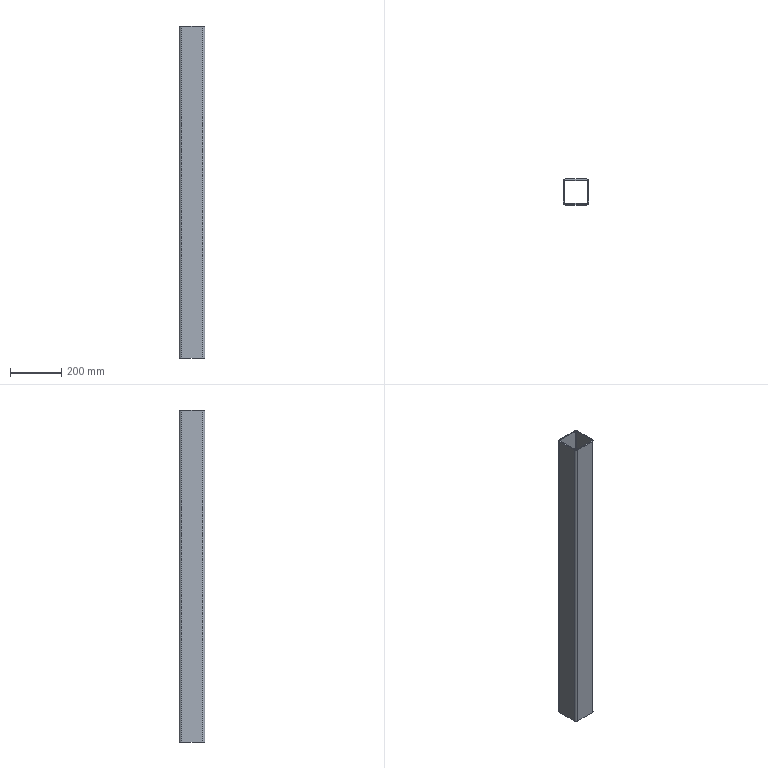Part | SolidWorks | features Extrusion 1 | 1 solid | 18 faces | box 100 x 100 x 1290 mm | volume 2367949 mm3 | plane 10 | cylinder 8 | commonest cylinder face diameters 10 x4 20 x4
STEP:
#1=CARTESIAN_POINT('',(-40.,50.,645.));
#2=VERTEX_POINT('',#1);
#3=CARTESIAN_POINT('',(-50.,40.,645.));
#4=VERTEX_POINT('',#3);
#5=CARTESIAN_POINT('',(-40.,40.,645.));
#6=DIRECTION('',(0.,0.,1.));
#7=DIRECTION('',(1.,0.,0.));
#8=AXIS2_PLACEMENT_3D('',#5,#6,#7);
#9=CIRCLE('',#8,10.);
#10=EDGE_CURVE('',#2,#4,#9,.T.);
#11=ORIENTED_EDGE('',*,*,#10,.T.);
#12=CARTESIAN_POINT('',(-50.,-40.,645.));
#13=VERTEX_POINT('',#12);
#14=CARTESIAN_POINT('',(-50.,40.,645.));
#15=DIRECTION('',(0.,-1.,0.));
#16=VECTOR('',#15,1000.);
#17=LINE('',#14,#16);
#18=EDGE_CURVE('',#4,#13,#17,.T.);
#19=ORIENTED_EDGE('',*,*,#18,.T.);
#20=CARTESIAN_POINT('',(-40.,-50.,645.));
#21=VERTEX_POINT('',#20);
#22=CARTESIAN_POINT('',(-40.,-40.,645.));
#23=DIRECTION('',(0.,0.,1.));
#24=DIRECTION('',(-1.,0.,0.));
#25=AXIS2_PLACEMENT_3D('',#22,#23,#24);
#26=CIRCLE('',#25,10.);
#27=EDGE_CURVE('',#13,#21,#26,.T.);
#28=ORIENTED_EDGE('',*,*,#27,.T.);
#29=CARTESIAN_POINT('',(40.,-50.,645.));
#30=VERTEX_POINT('',#29);
#31=CARTESIAN_POINT('',(40.,-50.,645.));
#32=DIRECTION('',(1.,0.,0.));
#33=VECTOR('',#32,1000.);
#34=LINE('',#31,#33);
#35=EDGE_CURVE('',#21,#30,#34,.T.);
#36=ORIENTED_EDGE('',*,*,#35,.T.);
#37=CARTESIAN_POINT('',(50.,-40.,645.));
#38=VERTEX_POINT('',#37);
#39=CARTESIAN_POINT('',(40.,-40.,645.));
#40=DIRECTION('',(0.,0.,1.));
#41=DIRECTION('',(1.,0.,0.));
#42=AXIS2_PLACEMENT_3D('',#39,#40,#41);
#43=CIRCLE('',#42,10.);
#44=EDGE_CURVE('',#30,#38,#43,.T.);
#45=ORIENTED_EDGE('',*,*,#44,.T.);
#46=CARTESIAN_POINT('',(50.,40.,645.));
#47=VERTEX_POINT('',#46);
#48=CARTESIAN_POINT('',(50.,-40.,645.));
#49=DIRECTION('',(0.,1.,0.));
#50=VECTOR('',#49,1000.);
#51=LINE('',#48,#50);
#52=EDGE_CURVE('',#38,#47,#51,.T.);
#53=ORIENTED_EDGE('',*,*,#52,.T.);
#54=CARTESIAN_POINT('',(40.,50.,645.));
#55=VERTEX_POINT('',#54);
#56=CARTESIAN_POINT('',(40.,40.,645.));
#57=DIRECTION('',(0.,0.,1.));
#58=DIRECTION('',(-1.,0.,0.));
#59=AXIS2_PLACEMENT_3D('',#56,#57,#58);
#60=CIRCLE('',#59,10.);
#61=EDGE_CURVE('',#47,#55,#60,.T.);
#62=ORIENTED_EDGE('',*,*,#61,.T.);
#63=CARTESIAN_POINT('',(0.,50.,645.));
#64=DIRECTION('',(-1.,0.,0.));
#65=VECTOR('',#64,1000.);
#66=LINE('',#63,#65);
#67=EDGE_CURVE('',#55,#2,#66,.T.);
#68=ORIENTED_EDGE('',*,*,#67,.T.);
#69=EDGE_LOOP('',(#11,#19,#28,#36,#45,#53,#62,#68));
#70=FACE_OUTER_BOUND('',#69,.T.);
#71=CARTESIAN_POINT('',(-45.,40.,645.));
#72=VERTEX_POINT('',#71);
#73=CARTESIAN_POINT('',(-45.,-40.,645.));
#74=VERTEX_POINT('',#73);
#75=CARTESIAN_POINT('',(-45.,40.,645.));
#76=DIRECTION('',(0.,-1.,0.));
#77=VECTOR('',#76,1000.);
#78=LINE('',#75,#77);
#79=EDGE_CURVE('',#72,#74,#78,.T.);
#80=ORIENTED_EDGE('',*,*,#79,.F.);
#81=CARTESIAN_POINT('',(-40.,45.,645.));
#82=VERTEX_POINT('',#81);
#83=CARTESIAN_POINT('',(-40.,40.,645.));
#84=DIRECTION('',(0.,0.,1.));
#85=DIRECTION('',(1.,0.,0.));
#86=AXIS2_PLACEMENT_3D('',#83,#84,#85);
#87=CIRCLE('',#86,5.);
#88=EDGE_CURVE('',#82,#72,#87,.T.);
#89=ORIENTED_EDGE('',*,*,#88,.F.);
#90=CARTESIAN_POINT('',(40.,45.,645.));
#91=VERTEX_POINT('',#90);
#92=CARTESIAN_POINT('',(0.,45.,645.));
#93=DIRECTION('',(-1.,0.,0.));
#94=VECTOR('',#93,1000.);
#95=LINE('',#92,#94);
#96=EDGE_CURVE('',#91,#82,#95,.T.);
#97=ORIENTED_EDGE('',*,*,#96,.F.);
#98=CARTESIAN_POINT('',(45.,40.,645.));
#99=VERTEX_POINT('',#98);
#100=CARTESIAN_POINT('',(40.,40.,645.));
#101=DIRECTION('',(0.,0.,1.));
#102=DIRECTION('',(-1.,0.,0.));
#103=AXIS2_PLACEMENT_3D('',#100,#101,#102);
#104=CIRCLE('',#103,5.);
#105=EDGE_CURVE('',#99,#91,#104,.T.);
#106=ORIENTED_EDGE('',*,*,#105,.F.);
#107=CARTESIAN_POINT('',(45.,-40.,645.));
#108=VERTEX_POINT('',#107);
#109=CARTESIAN_POINT('',(45.,-40.,645.));
#110=DIRECTION('',(0.,1.,0.));
#111=VECTOR('',#110,1000.);
#112=LINE('',#109,#111);
#113=EDGE_CURVE('',#108,#99,#112,.T.);
#114=ORIENTED_EDGE('',*,*,#113,.F.);
#115=CARTESIAN_POINT('',(40.,-45.,645.));
#116=VERTEX_POINT('',#115);
#117=CARTESIAN_POINT('',(40.,-40.,645.));
#118=DIRECTION('',(0.,0.,1.));
#119=DIRECTION('',(1.,0.,0.));
#120=AXIS2_PLACEMENT_3D('',#117,#118,#119);
#121=CIRCLE('',#120,5.);
#122=EDGE_CURVE('',#116,#108,#121,.T.);
#123=ORIENTED_EDGE('',*,*,#122,.F.);
#124=CARTESIAN_POINT('',(-40.,-45.,645.));
#125=VERTEX_POINT('',#124);
#126=CARTESIAN_POINT('',(40.,-45.,645.));
#127=DIRECTION('',(1.,0.,0.));
#128=VECTOR('',#127,1000.);
#129=LINE('',#126,#128);
#130=EDGE_CURVE('',#125,#116,#129,.T.);
#131=ORIENTED_EDGE('',*,*,#130,.F.);
#132=CARTESIAN_POINT('',(-40.,-40.,645.));
#133=DIRECTION('',(0.,0.,1.));
#134=DIRECTION('',(-1.,0.,0.));
#135=AXIS2_PLACEMENT_3D('',#132,#133,#134);
#136=CIRCLE('',#135,5.);
#137=EDGE_CURVE('',#74,#125,#136,.T.);
#138=ORIENTED_EDGE('',*,*,#137,.F.);
#139=EDGE_LOOP('',(#80,#89,#97,#106,#114,#123,#131,#138));
#140=FACE_BOUND('',#139,.T.);
#141=CARTESIAN_POINT('',(-40.,40.,645.));
#142=DIRECTION('',(0.,0.,1.));
#143=DIRECTION('',(1.,0.,0.));
#144=AXIS2_PLACEMENT_3D('',#141,#142,#143);
#145=PLANE('',#144);
#146=ADVANCED_FACE('',(#70,#140),#145,.T.);
#147=CARTESIAN_POINT('',(-40.,50.,-645.));
#148=VERTEX_POINT('',#147);
#149=CARTESIAN_POINT('',(-50.,40.,-645.));
#150=VERTEX_POINT('',#149);
#151=CARTESIAN_POINT('',(-40.,40.,-645.));
#152=DIRECTION('',(0.,0.,1.));
#153=DIRECTION('',(1.,0.,0.));
#154=AXIS2_PLACEMENT_3D('',#151,#152,#153);
#155=CIRCLE('',#154,10.);
#156=EDGE_CURVE('',#148,#150,#155,.T.);
#157=ORIENTED_EDGE('',*,*,#156,.F.);
#158=CARTESIAN_POINT('',(40.,50.,-645.));
#159=VERTEX_POINT('',#158);
#160=CARTESIAN_POINT('',(0.,50.,-645.));
#161=DIRECTION('',(-1.,0.,0.));
#162=VECTOR('',#161,1000.);
#163=LINE('',#160,#162);
#164=EDGE_CURVE('',#159,#148,#163,.T.);
#165=ORIENTED_EDGE('',*,*,#164,.F.);
#166=CARTESIAN_POINT('',(50.,40.,-645.));
#167=VERTEX_POINT('',#166);
#168=CARTESIAN_POINT('',(40.,40.,-645.));
#169=DIRECTION('',(0.,0.,1.));
#170=DIRECTION('',(-1.,0.,0.));
#171=AXIS2_PLACEMENT_3D('',#168,#169,#170);
#172=CIRCLE('',#171,10.);
#173=EDGE_CURVE('',#167,#159,#172,.T.);
#174=ORIENTED_EDGE('',*,*,#173,.F.);
#175=CARTESIAN_POINT('',(50.,-40.,-645.));
#176=VERTEX_POINT('',#175);
#177=CARTESIAN_POINT('',(50.,40.,-645.));
#178=DIRECTION('',(0.,1.,0.));
#179=VECTOR('',#178,1000.);
#180=LINE('',#177,#179);
#181=EDGE_CURVE('',#176,#167,#180,.T.);
#182=ORIENTED_EDGE('',*,*,#181,.F.);
#183=CARTESIAN_POINT('',(40.,-50.,-645.));
#184=VERTEX_POINT('',#183);
#185=CARTESIAN_POINT('',(40.,-40.,-645.));
#186=DIRECTION('',(0.,0.,1.));
#187=DIRECTION('',(1.,0.,0.));
#188=AXIS2_PLACEMENT_3D('',#185,#186,#187);
#189=CIRCLE('',#188,10.);
#190=EDGE_CURVE('',#184,#176,#189,.T.);
#191=ORIENTED_EDGE('',*,*,#190,.F.);
#192=CARTESIAN_POINT('',(-40.,-50.,-645.));
#193=VERTEX_POINT('',#192);
#194=CARTESIAN_POINT('',(40.,-50.,-645.));
#195=DIRECTION('',(1.,0.,0.));
#196=VECTOR('',#195,1000.);
#197=LINE('',#194,#196);
#198=EDGE_CURVE('',#193,#184,#197,.T.);
#199=ORIENTED_EDGE('',*,*,#198,.F.);
#200=CARTESIAN_POINT('',(-50.,-40.,-645.));
#201=VERTEX_POINT('',#200);
#202=CARTESIAN_POINT('',(-40.,-40.,-645.));
#203=DIRECTION('',(0.,0.,1.));
#204=DIRECTION('',(-1.,0.,0.));
#205=AXIS2_PLACEMENT_3D('',#202,#203,#204);
#206=CIRCLE('',#205,10.);
#207=EDGE_CURVE('',#201,#193,#206,.T.);
#208=ORIENTED_EDGE('',*,*,#207,.F.);
#209=CARTESIAN_POINT('',(-50.,-40.,-645.));
#210=DIRECTION('',(0.,-1.,0.));
#211=VECTOR('',#210,1000.);
#212=LINE('',#209,#211);
#213=EDGE_CURVE('',#150,#201,#212,.T.);
#214=ORIENTED_EDGE('',*,*,#213,.F.);
#215=EDGE_LOOP('',(#157,#165,#174,#182,#191,#199,#208,#214));
#216=FACE_OUTER_BOUND('',#215,.T.);
#217=CARTESIAN_POINT('',(-40.,45.,-645.));
#218=VERTEX_POINT('',#217);
#219=CARTESIAN_POINT('',(-45.,40.,-645.));
#220=VERTEX_POINT('',#219);
#221=CARTESIAN_POINT('',(-40.,40.,-645.));
#222=DIRECTION('',(0.,0.,1.));
#223=DIRECTION('',(1.,0.,0.));
#224=AXIS2_PLACEMENT_3D('',#221,#222,#223);
#225=CIRCLE('',#224,5.);
#226=EDGE_CURVE('',#218,#220,#225,.T.);
#227=ORIENTED_EDGE('',*,*,#226,.T.);
#228=CARTESIAN_POINT('',(-45.,-40.,-645.));
#229=VERTEX_POINT('',#228);
#230=CARTESIAN_POINT('',(-45.,-40.,-645.));
#231=DIRECTION('',(0.,-1.,0.));
#232=VECTOR('',#231,1000.);
#233=LINE('',#230,#232);
#234=EDGE_CURVE('',#220,#229,#233,.T.);
#235=ORIENTED_EDGE('',*,*,#234,.T.);
#236=CARTESIAN_POINT('',(-40.,-45.,-645.));
#237=VERTEX_POINT('',#236);
#238=CARTESIAN_POINT('',(-40.,-40.,-645.));
#239=DIRECTION('',(0.,0.,1.));
#240=DIRECTION('',(-1.,0.,0.));
#241=AXIS2_PLACEMENT_3D('',#238,#239,#240);
#242=CIRCLE('',#241,5.);
#243=EDGE_CURVE('',#229,#237,#242,.T.);
#244=ORIENTED_EDGE('',*,*,#243,.T.);
#245=CARTESIAN_POINT('',(40.,-45.,-645.));
#246=VERTEX_POINT('',#245);
#247=CARTESIAN_POINT('',(40.,-45.,-645.));
#248=DIRECTION('',(1.,0.,0.));
#249=VECTOR('',#248,1000.);
#250=LINE('',#247,#249);
#251=EDGE_CURVE('',#237,#246,#250,.T.);
#252=ORIENTED_EDGE('',*,*,#251,.T.);
#253=CARTESIAN_POINT('',(45.,-40.,-645.));
#254=VERTEX_POINT('',#253);
#255=CARTESIAN_POINT('',(40.,-40.,-645.));
#256=DIRECTION('',(0.,0.,1.));
#257=DIRECTION('',(1.,0.,0.));
#258=AXIS2_PLACEMENT_3D('',#255,#256,#257);
#259=CIRCLE('',#258,5.);
#260=EDGE_CURVE('',#246,#254,#259,.T.);
#261=ORIENTED_EDGE('',*,*,#260,.T.);
#262=CARTESIAN_POINT('',(45.,40.,-645.));
#263=VERTEX_POINT('',#262);
#264=CARTESIAN_POINT('',(45.,40.,-645.));
#265=DIRECTION('',(0.,1.,0.));
#266=VECTOR('',#265,1000.);
#267=LINE('',#264,#266);
#268=EDGE_CURVE('',#254,#263,#267,.T.);
#269=ORIENTED_EDGE('',*,*,#268,.T.);
#270=CARTESIAN_POINT('',(40.,45.,-645.));
#271=VERTEX_POINT('',#270);
#272=CARTESIAN_POINT('',(40.,40.,-645.));
#273=DIRECTION('',(0.,0.,1.));
#274=DIRECTION('',(-1.,0.,0.));
#275=AXIS2_PLACEMENT_3D('',#272,#273,#274);
#276=CIRCLE('',#275,5.);
#277=EDGE_CURVE('',#263,#271,#276,.T.);
#278=ORIENTED_EDGE('',*,*,#277,.T.);
#279=CARTESIAN_POINT('',(0.,45.,-645.));
#280=DIRECTION('',(-1.,0.,0.));
#281=VECTOR('',#280,1000.);
#282=LINE('',#279,#281);
#283=EDGE_CURVE('',#271,#218,#282,.T.);
#284=ORIENTED_EDGE('',*,*,#283,.T.);
#285=EDGE_LOOP('',(#227,#235,#244,#252,#261,#269,#278,#284));
#286=FACE_BOUND('',#285,.T.);
#287=CARTESIAN_POINT('',(-40.,40.,-645.));
#288=DIRECTION('',(0.,0.,1.));
#289=DIRECTION('',(1.,0.,0.));
#290=AXIS2_PLACEMENT_3D('',#287,#288,#289);
#291=PLANE('',#290);
#292=ADVANCED_FACE('',(#216,#286),#291,.F.);
#293=ORIENTED_EDGE('',*,*,#156,.T.);
#294=CARTESIAN_POINT('',(-50.,40.,645.));
#295=DIRECTION('',(0.,0.,-1.));
#296=VECTOR('',#295,1000.);
#297=LINE('',#294,#296);
#298=EDGE_CURVE('',#4,#150,#297,.T.);
#299=ORIENTED_EDGE('',*,*,#298,.F.);
#300=ORIENTED_EDGE('',*,*,#10,.F.);
#301=CARTESIAN_POINT('',(-40.,50.,645.));
#302=DIRECTION('',(0.,0.,-1.));
#303=VECTOR('',#302,1000.);
#304=LINE('',#301,#303);
#305=EDGE_CURVE('',#2,#148,#304,.T.);
#306=ORIENTED_EDGE('',*,*,#305,.T.);
#307=EDGE_LOOP('',(#293,#299,#300,#306));
#308=FACE_OUTER_BOUND('',#307,.T.);
#309=CARTESIAN_POINT('',(-40.,40.,645.));
#310=DIRECTION('',(0.,0.,-1.));
#311=DIRECTION('',(-1.,0.,0.));
#312=AXIS2_PLACEMENT_3D('',#309,#310,#311);
#313=CYLINDRICAL_SURFACE('',#312,10.);
#314=ADVANCED_FACE('',(#308),#313,.T.);
#315=ORIENTED_EDGE('',*,*,#213,.T.);
#316=CARTESIAN_POINT('',(-50.,-40.,645.));
#317=DIRECTION('',(0.,0.,-1.));
#318=VECTOR('',#317,1000.);
#319=LINE('',#316,#318);
#320=EDGE_CURVE('',#13,#201,#319,.T.);
#321=ORIENTED_EDGE('',*,*,#320,.F.);
#322=ORIENTED_EDGE('',*,*,#18,.F.);
#323=ORIENTED_EDGE('',*,*,#298,.T.);
#324=EDGE_LOOP('',(#315,#321,#322,#323));
#325=FACE_OUTER_BOUND('',#324,.T.);
#326=CARTESIAN_POINT('',(-50.,-40.,645.));
#327=DIRECTION('',(1.,0.,0.));
#328=DIRECTION('',(0.,0.,-1.));
#329=AXIS2_PLACEMENT_3D('',#326,#327,#328);
#330=PLANE('',#329);
#331=ADVANCED_FACE('',(#325),#330,.F.);
#332=ORIENTED_EDGE('',*,*,#207,.T.);
#333=CARTESIAN_POINT('',(-40.,-50.,645.));
#334=DIRECTION('',(0.,0.,-1.));
#335=VECTOR('',#334,1000.);
#336=LINE('',#333,#335);
#337=EDGE_CURVE('',#21,#193,#336,.T.);
#338=ORIENTED_EDGE('',*,*,#337,.F.);
#339=ORIENTED_EDGE('',*,*,#27,.F.);
#340=ORIENTED_EDGE('',*,*,#320,.T.);
#341=EDGE_LOOP('',(#332,#338,#339,#340));
#342=FACE_OUTER_BOUND('',#341,.T.);
#343=CARTESIAN_POINT('',(-40.,-40.,645.));
#344=DIRECTION('',(0.,0.,-1.));
#345=DIRECTION('',(-1.,0.,0.));
#346=AXIS2_PLACEMENT_3D('',#343,#344,#345);
#347=CYLINDRICAL_SURFACE('',#346,10.);
#348=ADVANCED_FACE('',(#342),#347,.T.);
#349=ORIENTED_EDGE('',*,*,#198,.T.);
#350=CARTESIAN_POINT('',(40.,-50.,645.));
#351=DIRECTION('',(0.,0.,-1.));
#352=VECTOR('',#351,1000.);
#353=LINE('',#350,#352);
#354=EDGE_CURVE('',#30,#184,#353,.T.);
#355=ORIENTED_EDGE('',*,*,#354,.F.);
#356=ORIENTED_EDGE('',*,*,#35,.F.);
#357=ORIENTED_EDGE('',*,*,#337,.T.);
#358=EDGE_LOOP('',(#349,#355,#356,#357));
#359=FACE_OUTER_BOUND('',#358,.T.);
#360=CARTESIAN_POINT('',(40.,-50.,645.));
#361=DIRECTION('',(0.,1.,0.));
#362=DIRECTION('',(-1.,0.,0.));
#363=AXIS2_PLACEMENT_3D('',#360,#361,#362);
#364=PLANE('',#363);
#365=ADVANCED_FACE('',(#359),#364,.F.);
#366=ORIENTED_EDGE('',*,*,#190,.T.);
#367=CARTESIAN_POINT('',(50.,-40.,645.));
#368=DIRECTION('',(0.,0.,-1.));
#369=VECTOR('',#368,1000.);
#370=LINE('',#367,#369);
#371=EDGE_CURVE('',#38,#176,#370,.T.);
#372=ORIENTED_EDGE('',*,*,#371,.F.);
#373=ORIENTED_EDGE('',*,*,#44,.F.);
#374=ORIENTED_EDGE('',*,*,#354,.T.);
#375=EDGE_LOOP('',(#366,#372,#373,#374));
#376=FACE_OUTER_BOUND('',#375,.T.);
#377=CARTESIAN_POINT('',(40.,-40.,645.));
#378=DIRECTION('',(0.,0.,-1.));
#379=DIRECTION('',(-1.,0.,0.));
#380=AXIS2_PLACEMENT_3D('',#377,#378,#379);
#381=CYLINDRICAL_SURFACE('',#380,10.);
#382=ADVANCED_FACE('',(#376),#381,.T.);
#383=ORIENTED_EDGE('',*,*,#181,.T.);
#384=CARTESIAN_POINT('',(50.,40.,645.));
#385=DIRECTION('',(0.,0.,-1.));
#386=VECTOR('',#385,1000.);
#387=LINE('',#384,#386);
#388=EDGE_CURVE('',#47,#167,#387,.T.);
#389=ORIENTED_EDGE('',*,*,#388,.F.);
#390=ORIENTED_EDGE('',*,*,#52,.F.);
#391=ORIENTED_EDGE('',*,*,#371,.T.);
#392=EDGE_LOOP('',(#383,#389,#390,#391));
#393=FACE_OUTER_BOUND('',#392,.T.);
#394=CARTESIAN_POINT('',(50.,40.,645.));
#395=DIRECTION('',(-1.,0.,0.));
#396=DIRECTION('',(0.,0.,1.));
#397=AXIS2_PLACEMENT_3D('',#394,#395,#396);
#398=PLANE('',#397);
#399=ADVANCED_FACE('',(#393),#398,.F.);
#400=ORIENTED_EDGE('',*,*,#173,.T.);
#401=CARTESIAN_POINT('',(40.,50.,645.));
#402=DIRECTION('',(0.,0.,-1.));
#403=VECTOR('',#402,1000.);
#404=LINE('',#401,#403);
#405=EDGE_CURVE('',#55,#159,#404,.T.);
#406=ORIENTED_EDGE('',*,*,#405,.F.);
#407=ORIENTED_EDGE('',*,*,#61,.F.);
#408=ORIENTED_EDGE('',*,*,#388,.T.);
#409=EDGE_LOOP('',(#400,#406,#407,#408));
#410=FACE_OUTER_BOUND('',#409,.T.);
#411=CARTESIAN_POINT('',(40.,40.,645.));
#412=DIRECTION('',(0.,0.,-1.));
#413=DIRECTION('',(-1.,0.,0.));
#414=AXIS2_PLACEMENT_3D('',#411,#412,#413);
#415=CYLINDRICAL_SURFACE('',#414,10.);
#416=ADVANCED_FACE('',(#410),#415,.T.);
#417=ORIENTED_EDGE('',*,*,#164,.T.);
#418=ORIENTED_EDGE('',*,*,#305,.F.);
#419=ORIENTED_EDGE('',*,*,#67,.F.);
#420=ORIENTED_EDGE('',*,*,#405,.T.);
#421=EDGE_LOOP('',(#417,#418,#419,#420));
#422=FACE_OUTER_BOUND('',#421,.T.);
#423=CARTESIAN_POINT('',(0.,50.,645.));
#424=DIRECTION('',(0.,-1.,0.));
#425=DIRECTION('',(0.,0.,-1.));
#426=AXIS2_PLACEMENT_3D('',#423,#424,#425);
#427=PLANE('',#426);
#428=ADVANCED_FACE('',(#422),#427,.F.);
#429=ORIENTED_EDGE('',*,*,#226,.F.);
#430=CARTESIAN_POINT('',(-40.,45.,645.));
#431=DIRECTION('',(0.,0.,-1.));
#432=VECTOR('',#431,1000.);
#433=LINE('',#430,#432);
#434=EDGE_CURVE('',#82,#218,#433,.T.);
#435=ORIENTED_EDGE('',*,*,#434,.F.);
#436=ORIENTED_EDGE('',*,*,#88,.T.);
#437=CARTESIAN_POINT('',(-45.,40.,645.));
#438=DIRECTION('',(0.,0.,-1.));
#439=VECTOR('',#438,1000.);
#440=LINE('',#437,#439);
#441=EDGE_CURVE('',#72,#220,#440,.T.);
#442=ORIENTED_EDGE('',*,*,#441,.T.);
#443=EDGE_LOOP('',(#429,#435,#436,#442));
#444=FACE_OUTER_BOUND('',#443,.T.);
#445=CARTESIAN_POINT('',(-40.,40.,645.));
#446=DIRECTION('',(0.,0.,-1.));
#447=DIRECTION('',(-1.,0.,0.));
#448=AXIS2_PLACEMENT_3D('',#445,#446,#447);
#449=CYLINDRICAL_SURFACE('',#448,5.);
#450=ADVANCED_FACE('',(#444),#449,.F.);
#451=ORIENTED_EDGE('',*,*,#234,.F.);
#452=ORIENTED_EDGE('',*,*,#441,.F.);
#453=ORIENTED_EDGE('',*,*,#79,.T.);
#454=CARTESIAN_POINT('',(-45.,-40.,645.));
#455=DIRECTION('',(0.,0.,-1.));
#456=VECTOR('',#455,1000.);
#457=LINE('',#454,#456);
#458=EDGE_CURVE('',#74,#229,#457,.T.);
#459=ORIENTED_EDGE('',*,*,#458,.T.);
#460=EDGE_LOOP('',(#451,#452,#453,#459));
#461=FACE_OUTER_BOUND('',#460,.T.);
#462=CARTESIAN_POINT('',(-45.,-40.,645.));
#463=DIRECTION('',(1.,0.,0.));
#464=DIRECTION('',(0.,1.,0.));
#465=AXIS2_PLACEMENT_3D('',#462,#463,#464);
#466=PLANE('',#465);
#467=ADVANCED_FACE('',(#461),#466,.T.);
#468=ORIENTED_EDGE('',*,*,#243,.F.);
#469=ORIENTED_EDGE('',*,*,#458,.F.);
#470=ORIENTED_EDGE('',*,*,#137,.T.);
#471=CARTESIAN_POINT('',(-40.,-45.,645.));
#472=DIRECTION('',(0.,0.,-1.));
#473=VECTOR('',#472,1000.);
#474=LINE('',#471,#473);
#475=EDGE_CURVE('',#125,#237,#474,.T.);
#476=ORIENTED_EDGE('',*,*,#475,.T.);
#477=EDGE_LOOP('',(#468,#469,#470,#476));
#478=FACE_OUTER_BOUND('',#477,.T.);
#479=CARTESIAN_POINT('',(-40.,-40.,645.));
#480=DIRECTION('',(0.,0.,-1.));
#481=DIRECTION('',(-1.,0.,0.));
#482=AXIS2_PLACEMENT_3D('',#479,#480,#481);
#483=CYLINDRICAL_SURFACE('',#482,5.);
#484=ADVANCED_FACE('',(#478),#483,.F.);
#485=ORIENTED_EDGE('',*,*,#251,.F.);
#486=ORIENTED_EDGE('',*,*,#475,.F.);
#487=ORIENTED_EDGE('',*,*,#130,.T.);
#488=CARTESIAN_POINT('',(40.,-45.,645.));
#489=DIRECTION('',(0.,0.,-1.));
#490=VECTOR('',#489,1000.);
#491=LINE('',#488,#490);
#492=EDGE_CURVE('',#116,#246,#491,.T.);
#493=ORIENTED_EDGE('',*,*,#492,.T.);
#494=EDGE_LOOP('',(#485,#486,#487,#493));
#495=FACE_OUTER_BOUND('',#494,.T.);
#496=CARTESIAN_POINT('',(40.,-45.,645.));
#497=DIRECTION('',(0.,1.,0.));
#498=DIRECTION('',(-1.,0.,0.));
#499=AXIS2_PLACEMENT_3D('',#496,#497,#498);
#500=PLANE('',#499);
#501=ADVANCED_FACE('',(#495),#500,.T.);
#502=ORIENTED_EDGE('',*,*,#260,.F.);
#503=ORIENTED_EDGE('',*,*,#492,.F.);
#504=ORIENTED_EDGE('',*,*,#122,.T.);
#505=CARTESIAN_POINT('',(45.,-40.,645.));
#506=DIRECTION('',(0.,0.,-1.));
#507=VECTOR('',#506,1000.);
#508=LINE('',#505,#507);
#509=EDGE_CURVE('',#108,#254,#508,.T.);
#510=ORIENTED_EDGE('',*,*,#509,.T.);
#511=EDGE_LOOP('',(#502,#503,#504,#510));
#512=FACE_OUTER_BOUND('',#511,.T.);
#513=CARTESIAN_POINT('',(40.,-40.,645.));
#514=DIRECTION('',(0.,0.,-1.));
#515=DIRECTION('',(-1.,0.,0.));
#516=AXIS2_PLACEMENT_3D('',#513,#514,#515);
#517=CYLINDRICAL_SURFACE('',#516,5.);
#518=ADVANCED_FACE('',(#512),#517,.F.);
#519=ORIENTED_EDGE('',*,*,#268,.F.);
#520=ORIENTED_EDGE('',*,*,#509,.F.);
#521=ORIENTED_EDGE('',*,*,#113,.T.);
#522=CARTESIAN_POINT('',(45.,40.,645.));
#523=DIRECTION('',(0.,0.,-1.));
#524=VECTOR('',#523,1000.);
#525=LINE('',#522,#524);
#526=EDGE_CURVE('',#99,#263,#525,.T.);
#527=ORIENTED_EDGE('',*,*,#526,.T.);
#528=EDGE_LOOP('',(#519,#520,#521,#527));
#529=FACE_OUTER_BOUND('',#528,.T.);
#530=CARTESIAN_POINT('',(45.,40.,645.));
#531=DIRECTION('',(-1.,0.,0.));
#532=DIRECTION('',(0.,0.,1.));
#533=AXIS2_PLACEMENT_3D('',#530,#531,#532);
#534=PLANE('',#533);
#535=ADVANCED_FACE('',(#529),#534,.T.);
#536=ORIENTED_EDGE('',*,*,#277,.F.);
#537=ORIENTED_EDGE('',*,*,#526,.F.);
#538=ORIENTED_EDGE('',*,*,#105,.T.);
#539=CARTESIAN_POINT('',(40.,45.,645.));
#540=DIRECTION('',(0.,0.,-1.));
#541=VECTOR('',#540,1000.);
#542=LINE('',#539,#541);
#543=EDGE_CURVE('',#91,#271,#542,.T.);
#544=ORIENTED_EDGE('',*,*,#543,.T.);
#545=EDGE_LOOP('',(#536,#537,#538,#544));
#546=FACE_OUTER_BOUND('',#545,.T.);
#547=CARTESIAN_POINT('',(40.,40.,645.));
#548=DIRECTION('',(0.,0.,-1.));
#549=DIRECTION('',(-1.,0.,0.));
#550=AXIS2_PLACEMENT_3D('',#547,#548,#549);
#551=CYLINDRICAL_SURFACE('',#550,5.);
#552=ADVANCED_FACE('',(#546),#551,.F.);
#553=ORIENTED_EDGE('',*,*,#283,.F.);
#554=ORIENTED_EDGE('',*,*,#543,.F.);
#555=ORIENTED_EDGE('',*,*,#96,.T.);
#556=ORIENTED_EDGE('',*,*,#434,.T.);
#557=EDGE_LOOP('',(#553,#554,#555,#556));
#558=FACE_OUTER_BOUND('',#557,.T.);
#559=CARTESIAN_POINT('',(0.,45.,645.));
#560=DIRECTION('',(0.,-1.,0.));
#561=DIRECTION('',(1.,0.,0.));
#562=AXIS2_PLACEMENT_3D('',#559,#560,#561);
#563=PLANE('',#562);
#564=ADVANCED_FACE('',(#558),#563,.T.);
#565=CLOSED_SHELL('',(#146,#292,#314,#331,#348,#365,#382,#399,#416,#428,#450,#467,#484,#501,#518,#535,#552,#564));
#566=MANIFOLD_SOLID_BREP('',#565);
#567=CARTESIAN_POINT('',(0.,0.,0.));
#568=DIRECTION('',(0.,0.,1.));
#569=DIRECTION('',(1.,0.,0.));
#570=AXIS2_PLACEMENT_3D('',#567,#568,#569);
#571=(LENGTH_UNIT()NAMED_UNIT(*)SI_UNIT(.MILLI.,.METRE.));
#572=UNCERTAINTY_MEASURE_WITH_UNIT(LENGTH_MEASURE(0.00001),#571,'','');
#573=(NAMED_UNIT(*)PLANE_ANGLE_UNIT()SI_UNIT($,.RADIAN.));
#574=(NAMED_UNIT(*)SI_UNIT($,.STERADIAN.)SOLID_ANGLE_UNIT());
#575=(GEOMETRIC_REPRESENTATION_CONTEXT(3)GLOBAL_UNCERTAINTY_ASSIGNED_CONTEXT((#572))GLOBAL_UNIT_ASSIGNED_CONTEXT((#571,#573,#574))REPRESENTATION_CONTEXT('',''));
#576=ADVANCED_BREP_SHAPE_REPRESENTATION('',(#566,#570),#575);